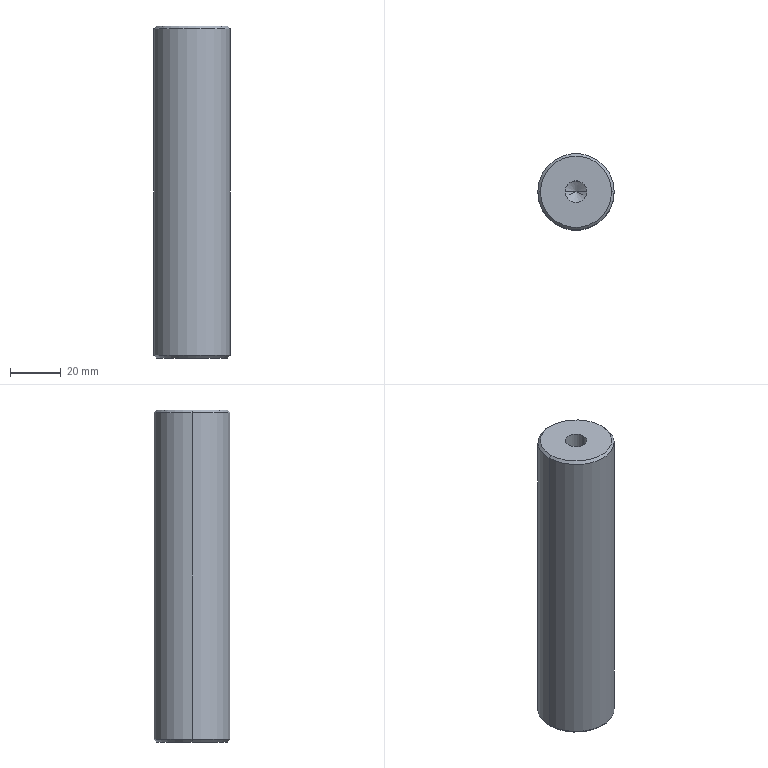Part | STEP file | LM-05-1254B_default | 1 solid | 16 faces | box 30 x 30 x 130.5 mm | volume 89786 mm3 | cone 8 | cylinder 6 | plane 2 | commonest cylinder face diameters 8.5 x4 30 x2
STEP:
#1=CARTESIAN_POINT('',(0.,0.,0.));
#2=DIRECTION('',(0.,0.,1.));
#3=DIRECTION('',(1.,0.,0.));
#4=AXIS2_PLACEMENT_3D('',#1,#2,#3);
#5=CARTESIAN_POINT('',(14.,0.,65.25));
#6=VERTEX_POINT('',#5);
#7=CARTESIAN_POINT('',(-14.,0.,65.25));
#8=VERTEX_POINT('',#7);
#9=CARTESIAN_POINT('',(0.,0.,65.25));
#10=DIRECTION('',(0.,0.,1.));
#11=DIRECTION('',(1.,0.,0.));
#12=AXIS2_PLACEMENT_3D('',#9,#10,#11);
#13=CIRCLE('',#12,14.);
#14=CARTESIAN_POINT('',(0.,0.,65.25));
#15=DIRECTION('',(0.,0.,-1.));
#16=DIRECTION('',(-1.,0.,0.));
#17=AXIS2_PLACEMENT_3D('',#14,#15,#16);
#18=CONICAL_SURFACE('',#17,14.,0.7854);
#19=CARTESIAN_POINT('',(3.142,0.));
#20=DIRECTION('',(-1.,0.));
#21=VECTOR('',#20,1.);
#22=LINE('',#19,#21);
#23=(GEOMETRIC_REPRESENTATION_CONTEXT(2)PARAMETRIC_REPRESENTATION_CONTEXT()REPRESENTATION_CONTEXT('',''));
#24=DEFINITIONAL_REPRESENTATION('',(#22),#23);
#25=PCURVE('',#18,#24);
#26=CARTESIAN_POINT('',(0.,0.,65.25));
#27=DIRECTION('',(0.,0.,1.));
#28=DIRECTION('',(1.,0.,0.));
#29=AXIS2_PLACEMENT_3D('',#26,#27,#28);
#30=PLANE('',#29);
#31=CARTESIAN_POINT('',(0.,0.));
#32=DIRECTION('',(1.,0.));
#33=AXIS2_PLACEMENT_2D('',#31,#32);
#34=CIRCLE('',#33,14.);
#35=(GEOMETRIC_REPRESENTATION_CONTEXT(2)PARAMETRIC_REPRESENTATION_CONTEXT()REPRESENTATION_CONTEXT('',''));
#36=DEFINITIONAL_REPRESENTATION('',(#34),#35);
#37=PCURVE('',#30,#36);
#38=SURFACE_CURVE('',#13,(#25,#37),.PCURVE_S1.);
#39=EDGE_CURVE('',#6,#8,#38,.T.);
#40=ORIENTED_EDGE('',*,*,#39,.F.);
#41=CARTESIAN_POINT('',(15.,0.,64.25));
#42=VERTEX_POINT('',#41);
#43=CARTESIAN_POINT('',(14.,0.,65.25));
#44=DIRECTION('',(0.7071,0.,-0.7071));
#45=VECTOR('',#44,1.);
#46=LINE('',#43,#45);
#47=CARTESIAN_POINT('',(3.142,0.));
#48=DIRECTION('',(0.,1.));
#49=VECTOR('',#48,1.);
#50=LINE('',#47,#49);
#51=(GEOMETRIC_REPRESENTATION_CONTEXT(2)PARAMETRIC_REPRESENTATION_CONTEXT()REPRESENTATION_CONTEXT('',''));
#52=DEFINITIONAL_REPRESENTATION('',(#50),#51);
#53=PCURVE('',#18,#52);
#54=CARTESIAN_POINT('',(0.,0.,65.25));
#55=DIRECTION('',(0.,0.,-1.));
#56=DIRECTION('',(-1.,0.,0.));
#57=AXIS2_PLACEMENT_3D('',#54,#55,#56);
#58=CONICAL_SURFACE('',#57,14.,0.7854);
#59=CARTESIAN_POINT('',(3.142,0.));
#60=DIRECTION('',(0.,1.));
#61=VECTOR('',#60,1.);
#62=LINE('',#59,#61);
#63=(GEOMETRIC_REPRESENTATION_CONTEXT(2)PARAMETRIC_REPRESENTATION_CONTEXT()REPRESENTATION_CONTEXT('',''));
#64=DEFINITIONAL_REPRESENTATION('',(#62),#63);
#65=PCURVE('',#58,#64);
#66=SURFACE_CURVE('',#46,(#53,#65),.PCURVE_S1.);
#67=EDGE_CURVE('',#6,#42,#66,.T.);
#68=ORIENTED_EDGE('',*,*,#67,.T.);
#69=CARTESIAN_POINT('',(-15.,0.,64.25));
#70=VERTEX_POINT('',#69);
#71=CARTESIAN_POINT('',(0.,0.,64.25));
#72=DIRECTION('',(0.,0.,-1.));
#73=DIRECTION('',(1.,0.,0.));
#74=AXIS2_PLACEMENT_3D('',#71,#72,#73);
#75=CIRCLE('',#74,15.);
#76=CARTESIAN_POINT('',(-3.142,1.));
#77=DIRECTION('',(1.,0.));
#78=VECTOR('',#77,1.);
#79=LINE('',#76,#78);
#80=(GEOMETRIC_REPRESENTATION_CONTEXT(2)PARAMETRIC_REPRESENTATION_CONTEXT()REPRESENTATION_CONTEXT('',''));
#81=DEFINITIONAL_REPRESENTATION('',(#79),#80);
#82=PCURVE('',#18,#81);
#83=CARTESIAN_POINT('',(0.,0.,65.25));
#84=DIRECTION('',(0.,0.,-1.));
#85=DIRECTION('',(-1.,0.,0.));
#86=AXIS2_PLACEMENT_3D('',#83,#84,#85);
#87=CYLINDRICAL_SURFACE('',#86,15.);
#88=CARTESIAN_POINT('',(-3.142,1.));
#89=DIRECTION('',(1.,0.));
#90=VECTOR('',#89,1.);
#91=LINE('',#88,#90);
#92=(GEOMETRIC_REPRESENTATION_CONTEXT(2)PARAMETRIC_REPRESENTATION_CONTEXT()REPRESENTATION_CONTEXT('',''));
#93=DEFINITIONAL_REPRESENTATION('',(#91),#92);
#94=PCURVE('',#87,#93);
#95=SURFACE_CURVE('',#75,(#82,#94),.PCURVE_S1.);
#96=EDGE_CURVE('',#70,#42,#95,.T.);
#97=ORIENTED_EDGE('',*,*,#96,.F.);
#98=CARTESIAN_POINT('',(-14.,0.,65.25));
#99=DIRECTION('',(-0.7071,0.,-0.7071));
#100=VECTOR('',#99,1.);
#101=LINE('',#98,#100);
#102=CARTESIAN_POINT('',(0.,0.));
#103=DIRECTION('',(0.,1.));
#104=VECTOR('',#103,1.);
#105=LINE('',#102,#104);
#106=(GEOMETRIC_REPRESENTATION_CONTEXT(2)PARAMETRIC_REPRESENTATION_CONTEXT()REPRESENTATION_CONTEXT('',''));
#107=DEFINITIONAL_REPRESENTATION('',(#105),#106);
#108=PCURVE('',#18,#107);
#109=CARTESIAN_POINT('',(6.283,0.));
#110=DIRECTION('',(0.,1.));
#111=VECTOR('',#110,1.);
#112=LINE('',#109,#111);
#113=(GEOMETRIC_REPRESENTATION_CONTEXT(2)PARAMETRIC_REPRESENTATION_CONTEXT()REPRESENTATION_CONTEXT('',''));
#114=DEFINITIONAL_REPRESENTATION('',(#112),#113);
#115=PCURVE('',#58,#114);
#116=SURFACE_CURVE('',#101,(#108,#115),.PCURVE_S1.);
#117=EDGE_CURVE('',#8,#70,#116,.T.);
#118=ORIENTED_EDGE('',*,*,#117,.F.);
#119=EDGE_LOOP('',(#40,#68,#97,#118));
#120=FACE_BOUND('',#119,.T.);
#121=ADVANCED_FACE('',(#120),#18,.T.);
#122=CARTESIAN_POINT('',(-14.,0.,-65.25));
#123=VERTEX_POINT('',#122);
#124=CARTESIAN_POINT('',(14.,0.,-65.25));
#125=VERTEX_POINT('',#124);
#126=CARTESIAN_POINT('',(0.,0.,-65.25));
#127=DIRECTION('',(0.,0.,-1.));
#128=DIRECTION('',(1.,0.,0.));
#129=AXIS2_PLACEMENT_3D('',#126,#127,#128);
#130=CIRCLE('',#129,14.);
#131=CARTESIAN_POINT('',(0.,0.,-64.25));
#132=DIRECTION('',(0.,0.,1.));
#133=DIRECTION('',(1.,0.,0.));
#134=AXIS2_PLACEMENT_3D('',#131,#132,#133);
#135=CONICAL_SURFACE('',#134,15.,0.7854);
#136=CARTESIAN_POINT('',(6.283,-1.));
#137=DIRECTION('',(-1.,0.));
#138=VECTOR('',#137,1.);
#139=LINE('',#136,#138);
#140=(GEOMETRIC_REPRESENTATION_CONTEXT(2)PARAMETRIC_REPRESENTATION_CONTEXT()REPRESENTATION_CONTEXT('',''));
#141=DEFINITIONAL_REPRESENTATION('',(#139),#140);
#142=PCURVE('',#135,#141);
#143=CARTESIAN_POINT('',(0.,0.,-65.25));
#144=DIRECTION('',(0.,0.,1.));
#145=DIRECTION('',(1.,0.,0.));
#146=AXIS2_PLACEMENT_3D('',#143,#144,#145);
#147=PLANE('',#146);
#148=CARTESIAN_POINT('',(14.,0.));
#149=CARTESIAN_POINT('',(14.,-24.249));
#150=CARTESIAN_POINT('',(-7.,-12.124));
#151=CARTESIAN_POINT('',(-28.,0.));
#152=CARTESIAN_POINT('',(-7.,12.124));
#153=CARTESIAN_POINT('',(14.,24.249));
#154=CARTESIAN_POINT('',(14.,0.));
#155=(BOUNDED_CURVE()B_SPLINE_CURVE(2,(#148,#149,#150,#151,#152,#153,#154),.UNSPECIFIED.,.T.,.F.)B_SPLINE_CURVE_WITH_KNOTS((1,2,2,2,2,1),(-2.094,0.,2.094,4.189,6.283,8.378),.UNSPECIFIED.)CURVE()GEOMETRIC_REPRESENTATION_ITEM()RATIONAL_B_SPLINE_CURVE((1.,0.5,1.,0.5,1.,0.5,1.))REPRESENTATION_ITEM(''));
#156=(GEOMETRIC_REPRESENTATION_CONTEXT(2)PARAMETRIC_REPRESENTATION_CONTEXT()REPRESENTATION_CONTEXT('',''));
#157=DEFINITIONAL_REPRESENTATION('',(#155),#156);
#158=PCURVE('',#147,#157);
#159=SURFACE_CURVE('',#130,(#142,#158),.PCURVE_S1.);
#160=EDGE_CURVE('',#123,#125,#159,.T.);
#161=ORIENTED_EDGE('',*,*,#160,.F.);
#162=CARTESIAN_POINT('',(-15.,0.,-64.25));
#163=VERTEX_POINT('',#162);
#164=CARTESIAN_POINT('',(-15.,0.,-64.25));
#165=DIRECTION('',(-0.7071,0.,0.7071));
#166=VECTOR('',#165,1.);
#167=LINE('',#164,#166);
#168=CARTESIAN_POINT('',(3.142,0.));
#169=DIRECTION('',(0.,1.));
#170=VECTOR('',#169,1.);
#171=LINE('',#168,#170);
#172=(GEOMETRIC_REPRESENTATION_CONTEXT(2)PARAMETRIC_REPRESENTATION_CONTEXT()REPRESENTATION_CONTEXT('',''));
#173=DEFINITIONAL_REPRESENTATION('',(#171),#172);
#174=PCURVE('',#135,#173);
#175=CARTESIAN_POINT('',(0.,0.,-64.25));
#176=DIRECTION('',(0.,0.,1.));
#177=DIRECTION('',(1.,0.,0.));
#178=AXIS2_PLACEMENT_3D('',#175,#176,#177);
#179=CONICAL_SURFACE('',#178,15.,0.7854);
#180=CARTESIAN_POINT('',(3.142,0.));
#181=DIRECTION('',(0.,1.));
#182=VECTOR('',#181,1.);
#183=LINE('',#180,#182);
#184=(GEOMETRIC_REPRESENTATION_CONTEXT(2)PARAMETRIC_REPRESENTATION_CONTEXT()REPRESENTATION_CONTEXT('',''));
#185=DEFINITIONAL_REPRESENTATION('',(#183),#184);
#186=PCURVE('',#179,#185);
#187=SURFACE_CURVE('',#167,(#174,#186),.PCURVE_S1.);
#188=EDGE_CURVE('',#123,#163,#187,.T.);
#189=ORIENTED_EDGE('',*,*,#188,.T.);
#190=CARTESIAN_POINT('',(15.,0.,-64.25));
#191=VERTEX_POINT('',#190);
#192=CARTESIAN_POINT('',(0.,0.,-64.25));
#193=DIRECTION('',(0.,0.,1.));
#194=DIRECTION('',(1.,0.,0.));
#195=AXIS2_PLACEMENT_3D('',#192,#193,#194);
#196=CIRCLE('',#195,15.);
#197=CARTESIAN_POINT('',(0.,0.));
#198=DIRECTION('',(1.,0.));
#199=VECTOR('',#198,1.);
#200=LINE('',#197,#199);
#201=(GEOMETRIC_REPRESENTATION_CONTEXT(2)PARAMETRIC_REPRESENTATION_CONTEXT()REPRESENTATION_CONTEXT('',''));
#202=DEFINITIONAL_REPRESENTATION('',(#200),#201);
#203=PCURVE('',#135,#202);
#204=CARTESIAN_POINT('',(3.142,129.5));
#205=DIRECTION('',(-1.,0.));
#206=VECTOR('',#205,1.);
#207=LINE('',#204,#206);
#208=(GEOMETRIC_REPRESENTATION_CONTEXT(2)PARAMETRIC_REPRESENTATION_CONTEXT()REPRESENTATION_CONTEXT('',''));
#209=DEFINITIONAL_REPRESENTATION('',(#207),#208);
#210=PCURVE('',#87,#209);
#211=SURFACE_CURVE('',#196,(#203,#210),.PCURVE_S1.);
#212=EDGE_CURVE('',#191,#163,#211,.T.);
#213=ORIENTED_EDGE('',*,*,#212,.F.);
#214=CARTESIAN_POINT('',(15.,0.,-64.25));
#215=DIRECTION('',(0.7071,0.,0.7071));
#216=VECTOR('',#215,1.);
#217=LINE('',#214,#216);
#218=CARTESIAN_POINT('',(0.,0.));
#219=DIRECTION('',(0.,1.));
#220=VECTOR('',#219,1.);
#221=LINE('',#218,#220);
#222=(GEOMETRIC_REPRESENTATION_CONTEXT(2)PARAMETRIC_REPRESENTATION_CONTEXT()REPRESENTATION_CONTEXT('',''));
#223=DEFINITIONAL_REPRESENTATION('',(#221),#222);
#224=PCURVE('',#135,#223);
#225=CARTESIAN_POINT('',(6.283,0.));
#226=DIRECTION('',(0.,1.));
#227=VECTOR('',#226,1.);
#228=LINE('',#225,#227);
#229=(GEOMETRIC_REPRESENTATION_CONTEXT(2)PARAMETRIC_REPRESENTATION_CONTEXT()REPRESENTATION_CONTEXT('',''));
#230=DEFINITIONAL_REPRESENTATION('',(#228),#229);
#231=PCURVE('',#179,#230);
#232=SURFACE_CURVE('',#217,(#224,#231),.PCURVE_S1.);
#233=EDGE_CURVE('',#125,#191,#232,.T.);
#234=ORIENTED_EDGE('',*,*,#233,.F.);
#235=EDGE_LOOP('',(#161,#189,#213,#234));
#236=FACE_BOUND('',#235,.T.);
#237=ADVANCED_FACE('',(#236),#135,.T.);
#238=CARTESIAN_POINT('',(-4.25,0.,-45.25));
#239=VERTEX_POINT('',#238);
#240=CARTESIAN_POINT('',(-4.25,0.,-65.25));
#241=VERTEX_POINT('',#240);
#242=CARTESIAN_POINT('',(-4.25,0.,-65.25));
#243=DIRECTION('',(0.,0.,-1.));
#244=VECTOR('',#243,1.);
#245=LINE('',#242,#244);
#246=CARTESIAN_POINT('',(0.,0.,-65.25));
#247=DIRECTION('',(0.,0.,-1.));
#248=DIRECTION('',(-1.,0.,0.));
#249=AXIS2_PLACEMENT_3D('',#246,#247,#248);
#250=CYLINDRICAL_SURFACE('',#249,4.25);
#251=CARTESIAN_POINT('',(6.283,0.));
#252=DIRECTION('',(0.,1.));
#253=VECTOR('',#252,1.);
#254=LINE('',#251,#253);
#255=(GEOMETRIC_REPRESENTATION_CONTEXT(2)PARAMETRIC_REPRESENTATION_CONTEXT()REPRESENTATION_CONTEXT('',''));
#256=DEFINITIONAL_REPRESENTATION('',(#254),#255);
#257=PCURVE('',#250,#256);
#258=CARTESIAN_POINT('',(0.,0.,-65.25));
#259=DIRECTION('',(0.,0.,-1.));
#260=DIRECTION('',(-1.,0.,0.));
#261=AXIS2_PLACEMENT_3D('',#258,#259,#260);
#262=CYLINDRICAL_SURFACE('',#261,4.25);
#263=CARTESIAN_POINT('',(0.,0.));
#264=DIRECTION('',(0.,1.));
#265=VECTOR('',#264,1.);
#266=LINE('',#263,#265);
#267=(GEOMETRIC_REPRESENTATION_CONTEXT(2)PARAMETRIC_REPRESENTATION_CONTEXT()REPRESENTATION_CONTEXT('',''));
#268=DEFINITIONAL_REPRESENTATION('',(#266),#267);
#269=PCURVE('',#262,#268);
#270=SURFACE_CURVE('',#245,(#257,#269),.PCURVE_S1.);
#271=EDGE_CURVE('',#239,#241,#270,.T.);
#272=ORIENTED_EDGE('',*,*,#271,.T.);
#273=CARTESIAN_POINT('',(4.25,0.,-65.25));
#274=VERTEX_POINT('',#273);
#275=CARTESIAN_POINT('',(0.,0.,-65.25));
#276=DIRECTION('',(0.,0.,-1.));
#277=DIRECTION('',(-1.,0.,0.));
#278=AXIS2_PLACEMENT_3D('',#275,#276,#277);
#279=CIRCLE('',#278,4.25);
#280=CARTESIAN_POINT('',(0.,0.));
#281=DIRECTION('',(1.,0.));
#282=VECTOR('',#281,1.);
#283=LINE('',#280,#282);
#284=(GEOMETRIC_REPRESENTATION_CONTEXT(2)PARAMETRIC_REPRESENTATION_CONTEXT()REPRESENTATION_CONTEXT('',''));
#285=DEFINITIONAL_REPRESENTATION('',(#283),#284);
#286=PCURVE('',#250,#285);
#287=CARTESIAN_POINT('',(-4.25,0.));
#288=CARTESIAN_POINT('',(-4.25,7.361));
#289=CARTESIAN_POINT('',(2.125,3.681));
#290=CARTESIAN_POINT('',(8.5,0.));
#291=CARTESIAN_POINT('',(2.125,-3.681));
#292=CARTESIAN_POINT('',(-4.25,-7.361));
#293=CARTESIAN_POINT('',(-4.25,0.));
#294=(BOUNDED_CURVE()B_SPLINE_CURVE(2,(#287,#288,#289,#290,#291,#292,#293),.UNSPECIFIED.,.T.,.F.)B_SPLINE_CURVE_WITH_KNOTS((1,2,2,2,2,1),(-2.094,0.,2.094,4.189,6.283,8.378),.UNSPECIFIED.)CURVE()GEOMETRIC_REPRESENTATION_ITEM()RATIONAL_B_SPLINE_CURVE((1.,0.5,1.,0.5,1.,0.5,1.))REPRESENTATION_ITEM(''));
#295=(GEOMETRIC_REPRESENTATION_CONTEXT(2)PARAMETRIC_REPRESENTATION_CONTEXT()REPRESENTATION_CONTEXT('',''));
#296=DEFINITIONAL_REPRESENTATION('',(#294),#295);
#297=PCURVE('',#147,#296);
#298=SURFACE_CURVE('',#279,(#286,#297),.PCURVE_S1.);
#299=EDGE_CURVE('',#274,#241,#298,.T.);
#300=ORIENTED_EDGE('',*,*,#299,.F.);
#301=CARTESIAN_POINT('',(4.25,0.,-45.25));
#302=VERTEX_POINT('',#301);
#303=CARTESIAN_POINT('',(4.25,0.,-65.25));
#304=DIRECTION('',(0.,0.,-1.));
#305=VECTOR('',#304,1.);
#306=LINE('',#303,#305);
#307=CARTESIAN_POINT('',(3.142,0.));
#308=DIRECTION('',(0.,1.));
#309=VECTOR('',#308,1.);
#310=LINE('',#307,#309);
#311=(GEOMETRIC_REPRESENTATION_CONTEXT(2)PARAMETRIC_REPRESENTATION_CONTEXT()REPRESENTATION_CONTEXT('',''));
#312=DEFINITIONAL_REPRESENTATION('',(#310),#311);
#313=PCURVE('',#250,#312);
#314=CARTESIAN_POINT('',(3.142,0.));
#315=DIRECTION('',(0.,1.));
#316=VECTOR('',#315,1.);
#317=LINE('',#314,#316);
#318=(GEOMETRIC_REPRESENTATION_CONTEXT(2)PARAMETRIC_REPRESENTATION_CONTEXT()REPRESENTATION_CONTEXT('',''));
#319=DEFINITIONAL_REPRESENTATION('',(#317),#318);
#320=PCURVE('',#262,#319);
#321=SURFACE_CURVE('',#306,(#313,#320),.PCURVE_S1.);
#322=EDGE_CURVE('',#302,#274,#321,.T.);
#323=ORIENTED_EDGE('',*,*,#322,.F.);
#324=CARTESIAN_POINT('',(0.,0.,-45.25));
#325=DIRECTION('',(0.,0.,-1.));
#326=DIRECTION('',(-1.,0.,0.));
#327=AXIS2_PLACEMENT_3D('',#324,#325,#326);
#328=CIRCLE('',#327,4.25);
#329=CARTESIAN_POINT('',(0.,-20.));
#330=DIRECTION('',(1.,0.));
#331=VECTOR('',#330,1.);
#332=LINE('',#329,#331);
#333=(GEOMETRIC_REPRESENTATION_CONTEXT(2)PARAMETRIC_REPRESENTATION_CONTEXT()REPRESENTATION_CONTEXT('',''));
#334=DEFINITIONAL_REPRESENTATION('',(#332),#333);
#335=PCURVE('',#250,#334);
#336=CARTESIAN_POINT('',(0.,0.,-45.25));
#337=DIRECTION('',(0.,0.,-1.));
#338=DIRECTION('',(-1.,0.,0.));
#339=AXIS2_PLACEMENT_3D('',#336,#337,#338);
#340=CONICAL_SURFACE('',#339,4.25,1.03);
#341=CARTESIAN_POINT('',(0.,0.));
#342=DIRECTION('',(1.,0.));
#343=VECTOR('',#342,1.);
#344=LINE('',#341,#343);
#345=(GEOMETRIC_REPRESENTATION_CONTEXT(2)PARAMETRIC_REPRESENTATION_CONTEXT()REPRESENTATION_CONTEXT('',''));
#346=DEFINITIONAL_REPRESENTATION('',(#344),#345);
#347=PCURVE('',#340,#346);
#348=SURFACE_CURVE('',#328,(#335,#347),.PCURVE_S1.);
#349=EDGE_CURVE('',#302,#239,#348,.T.);
#350=ORIENTED_EDGE('',*,*,#349,.T.);
#351=EDGE_LOOP('',(#272,#300,#323,#350));
#352=FACE_BOUND('',#351,.F.);
#353=ADVANCED_FACE('',(#352),#250,.F.);
#354=ORIENTED_EDGE('',*,*,#349,.F.);
#355=CARTESIAN_POINT('',(0.,0.,-42.696));
#356=VERTEX_POINT('',#355);
#357=CARTESIAN_POINT('',(4.25,0.,-45.25));
#358=DIRECTION('',(0.8572,0.,-0.515));
#359=VECTOR('',#358,1.);
#360=LINE('',#357,#359);
#361=CARTESIAN_POINT('',(3.142,0.));
#362=DIRECTION('',(0.,1.));
#363=VECTOR('',#362,1.);
#364=LINE('',#361,#363);
#365=(GEOMETRIC_REPRESENTATION_CONTEXT(2)PARAMETRIC_REPRESENTATION_CONTEXT()REPRESENTATION_CONTEXT('',''));
#366=DEFINITIONAL_REPRESENTATION('',(#364),#365);
#367=PCURVE('',#340,#366);
#368=CARTESIAN_POINT('',(0.,0.,-45.25));
#369=DIRECTION('',(0.,0.,-1.));
#370=DIRECTION('',(-1.,0.,0.));
#371=AXIS2_PLACEMENT_3D('',#368,#369,#370);
#372=CONICAL_SURFACE('',#371,4.25,1.03);
#373=CARTESIAN_POINT('',(3.142,0.));
#374=DIRECTION('',(0.,1.));
#375=VECTOR('',#374,1.);
#376=LINE('',#373,#375);
#377=(GEOMETRIC_REPRESENTATION_CONTEXT(2)PARAMETRIC_REPRESENTATION_CONTEXT()REPRESENTATION_CONTEXT('',''));
#378=DEFINITIONAL_REPRESENTATION('',(#376),#377);
#379=PCURVE('',#372,#378);
#380=SURFACE_CURVE('',#360,(#367,#379),.PCURVE_S1.);
#381=EDGE_CURVE('',#356,#302,#380,.T.);
#382=ORIENTED_EDGE('',*,*,#381,.F.);
#383=CARTESIAN_POINT('',(-4.25,0.,-45.25));
#384=DIRECTION('',(-0.8572,0.,-0.515));
#385=VECTOR('',#384,1.);
#386=LINE('',#383,#385);
#387=CARTESIAN_POINT('',(6.283,0.));
#388=DIRECTION('',(0.,1.));
#389=VECTOR('',#388,1.);
#390=LINE('',#387,#389);
#391=(GEOMETRIC_REPRESENTATION_CONTEXT(2)PARAMETRIC_REPRESENTATION_CONTEXT()REPRESENTATION_CONTEXT('',''));
#392=DEFINITIONAL_REPRESENTATION('',(#390),#391);
#393=PCURVE('',#340,#392);
#394=CARTESIAN_POINT('',(0.,0.));
#395=DIRECTION('',(0.,1.));
#396=VECTOR('',#395,1.);
#397=LINE('',#394,#396);
#398=(GEOMETRIC_REPRESENTATION_CONTEXT(2)PARAMETRIC_REPRESENTATION_CONTEXT()REPRESENTATION_CONTEXT('',''));
#399=DEFINITIONAL_REPRESENTATION('',(#397),#398);
#400=PCURVE('',#372,#399);
#401=SURFACE_CURVE('',#386,(#393,#400),.PCURVE_S1.);
#402=EDGE_CURVE('',#356,#239,#401,.T.);
#403=ORIENTED_EDGE('',*,*,#402,.T.);
#404=EDGE_LOOP('',(#354,#382,#403));
#405=FACE_BOUND('',#404,.F.);
#406=ADVANCED_FACE('',(#405),#340,.F.);
#407=CARTESIAN_POINT('',(4.25,0.,45.25));
#408=VERTEX_POINT('',#407);
#409=CARTESIAN_POINT('',(4.25,0.,65.25));
#410=VERTEX_POINT('',#409);
#411=CARTESIAN_POINT('',(4.25,0.,65.25));
#412=DIRECTION('',(0.,0.,1.));
#413=VECTOR('',#412,1.);
#414=LINE('',#411,#413);
#415=CARTESIAN_POINT('',(0.,0.,65.25));
#416=DIRECTION('',(0.,0.,1.));
#417=DIRECTION('',(1.,0.,0.));
#418=AXIS2_PLACEMENT_3D('',#415,#416,#417);
#419=CYLINDRICAL_SURFACE('',#418,4.25);
#420=CARTESIAN_POINT('',(6.283,0.));
#421=DIRECTION('',(0.,1.));
#422=VECTOR('',#421,1.);
#423=LINE('',#420,#422);
#424=(GEOMETRIC_REPRESENTATION_CONTEXT(2)PARAMETRIC_REPRESENTATION_CONTEXT()REPRESENTATION_CONTEXT('',''));
#425=DEFINITIONAL_REPRESENTATION('',(#423),#424);
#426=PCURVE('',#419,#425);
#427=CARTESIAN_POINT('',(0.,0.,65.25));
#428=DIRECTION('',(0.,0.,1.));
#429=DIRECTION('',(1.,0.,0.));
#430=AXIS2_PLACEMENT_3D('',#427,#428,#429);
#431=CYLINDRICAL_SURFACE('',#430,4.25);
#432=CARTESIAN_POINT('',(0.,0.));
#433=DIRECTION('',(0.,1.));
#434=VECTOR('',#433,1.);
#435=LINE('',#432,#434);
#436=(GEOMETRIC_REPRESENTATION_CONTEXT(2)PARAMETRIC_REPRESENTATION_CONTEXT()REPRESENTATION_CONTEXT('',''));
#437=DEFINITIONAL_REPRESENTATION('',(#435),#436);
#438=PCURVE('',#431,#437);
#439=SURFACE_CURVE('',#414,(#426,#438),.PCURVE_S1.);
#440=EDGE_CURVE('',#408,#410,#439,.T.);
#441=ORIENTED_EDGE('',*,*,#440,.T.);
#442=CARTESIAN_POINT('',(-4.25,0.,65.25));
#443=VERTEX_POINT('',#442);
#444=CARTESIAN_POINT('',(0.,0.,65.25));
#445=DIRECTION('',(0.,0.,1.));
#446=DIRECTION('',(1.,0.,0.));
#447=AXIS2_PLACEMENT_3D('',#444,#445,#446);
#448=CIRCLE('',#447,4.25);
#449=CARTESIAN_POINT('',(0.,0.));
#450=DIRECTION('',(1.,0.));
#451=VECTOR('',#450,1.);
#452=LINE('',#449,#451);
#453=(GEOMETRIC_REPRESENTATION_CONTEXT(2)PARAMETRIC_REPRESENTATION_CONTEXT()REPRESENTATION_CONTEXT('',''));
#454=DEFINITIONAL_REPRESENTATION('',(#452),#453);
#455=PCURVE('',#419,#454);
#456=CARTESIAN_POINT('',(0.,0.));
#457=DIRECTION('',(1.,0.));
#458=AXIS2_PLACEMENT_2D('',#456,#457);
#459=CIRCLE('',#458,4.25);
#460=(GEOMETRIC_REPRESENTATION_CONTEXT(2)PARAMETRIC_REPRESENTATION_CONTEXT()REPRESENTATION_CONTEXT('',''));
#461=DEFINITIONAL_REPRESENTATION('',(#459),#460);
#462=PCURVE('',#30,#461);
#463=SURFACE_CURVE('',#448,(#455,#462),.PCURVE_S1.);
#464=EDGE_CURVE('',#443,#410,#463,.T.);
#465=ORIENTED_EDGE('',*,*,#464,.F.);
#466=CARTESIAN_POINT('',(-4.25,0.,45.25));
#467=VERTEX_POINT('',#466);
#468=CARTESIAN_POINT('',(-4.25,0.,65.25));
#469=DIRECTION('',(0.,0.,1.));
#470=VECTOR('',#469,1.);
#471=LINE('',#468,#470);
#472=CARTESIAN_POINT('',(3.142,0.));
#473=DIRECTION('',(0.,1.));
#474=VECTOR('',#473,1.);
#475=LINE('',#472,#474);
#476=(GEOMETRIC_REPRESENTATION_CONTEXT(2)PARAMETRIC_REPRESENTATION_CONTEXT()REPRESENTATION_CONTEXT('',''));
#477=DEFINITIONAL_REPRESENTATION('',(#475),#476);
#478=PCURVE('',#419,#477);
#479=CARTESIAN_POINT('',(3.142,0.));
#480=DIRECTION('',(0.,1.));
#481=VECTOR('',#480,1.);
#482=LINE('',#479,#481);
#483=(GEOMETRIC_REPRESENTATION_CONTEXT(2)PARAMETRIC_REPRESENTATION_CONTEXT()REPRESENTATION_CONTEXT('',''));
#484=DEFINITIONAL_REPRESENTATION('',(#482),#483);
#485=PCURVE('',#431,#484);
#486=SURFACE_CURVE('',#471,(#478,#485),.PCURVE_S1.);
#487=EDGE_CURVE('',#467,#443,#486,.T.);
#488=ORIENTED_EDGE('',*,*,#487,.F.);
#489=CARTESIAN_POINT('',(0.,0.,45.25));
#490=DIRECTION('',(0.,0.,1.));
#491=DIRECTION('',(1.,0.,0.));
#492=AXIS2_PLACEMENT_3D('',#489,#490,#491);
#493=CIRCLE('',#492,4.25);
#494=CARTESIAN_POINT('',(0.,-20.));
#495=DIRECTION('',(1.,0.));
#496=VECTOR('',#495,1.);
#497=LINE('',#494,#496);
#498=(GEOMETRIC_REPRESENTATION_CONTEXT(2)PARAMETRIC_REPRESENTATION_CONTEXT()REPRESENTATION_CONTEXT('',''));
#499=DEFINITIONAL_REPRESENTATION('',(#497),#498);
#500=PCURVE('',#419,#499);
#501=CARTESIAN_POINT('',(0.,0.,45.25));
#502=DIRECTION('',(0.,0.,1.));
#503=DIRECTION('',(1.,0.,0.));
#504=AXIS2_PLACEMENT_3D('',#501,#502,#503);
#505=CONICAL_SURFACE('',#504,4.25,1.03);
#506=CARTESIAN_POINT('',(0.,0.));
#507=DIRECTION('',(1.,0.));
#508=VECTOR('',#507,1.);
#509=LINE('',#506,#508);
#510=(GEOMETRIC_REPRESENTATION_CONTEXT(2)PARAMETRIC_REPRESENTATION_CONTEXT()REPRESENTATION_CONTEXT('',''));
#511=DEFINITIONAL_REPRESENTATION('',(#509),#510);
#512=PCURVE('',#505,#511);
#513=SURFACE_CURVE('',#493,(#500,#512),.PCURVE_S1.);
#514=EDGE_CURVE('',#467,#408,#513,.T.);
#515=ORIENTED_EDGE('',*,*,#514,.T.);
#516=EDGE_LOOP('',(#441,#465,#488,#515));
#517=FACE_BOUND('',#516,.F.);
#518=ADVANCED_FACE('',(#517),#419,.F.);
#519=ORIENTED_EDGE('',*,*,#514,.F.);
#520=CARTESIAN_POINT('',(0.,0.,42.696));
#521=VERTEX_POINT('',#520);
#522=CARTESIAN_POINT('',(-4.25,0.,45.25));
#523=DIRECTION('',(-0.8572,0.,0.515));
#524=VECTOR('',#523,1.);
#525=LINE('',#522,#524);
#526=CARTESIAN_POINT('',(3.142,0.));
#527=DIRECTION('',(0.,1.));
#528=VECTOR('',#527,1.);
#529=LINE('',#526,#528);
#530=(GEOMETRIC_REPRESENTATION_CONTEXT(2)PARAMETRIC_REPRESENTATION_CONTEXT()REPRESENTATION_CONTEXT('',''));
#531=DEFINITIONAL_REPRESENTATION('',(#529),#530);
#532=PCURVE('',#505,#531);
#533=CARTESIAN_POINT('',(0.,0.,45.25));
#534=DIRECTION('',(0.,0.,1.));
#535=DIRECTION('',(1.,0.,0.));
#536=AXIS2_PLACEMENT_3D('',#533,#534,#535);
#537=CONICAL_SURFACE('',#536,4.25,1.03);
#538=CARTESIAN_POINT('',(3.142,0.));
#539=DIRECTION('',(0.,1.));
#540=VECTOR('',#539,1.);
#541=LINE('',#538,#540);
#542=(GEOMETRIC_REPRESENTATION_CONTEXT(2)PARAMETRIC_REPRESENTATION_CONTEXT()REPRESENTATION_CONTEXT('',''));
#543=DEFINITIONAL_REPRESENTATION('',(#541),#542);
#544=PCURVE('',#537,#543);
#545=SURFACE_CURVE('',#525,(#532,#544),.PCURVE_S1.);
#546=EDGE_CURVE('',#521,#467,#545,.T.);
#547=ORIENTED_EDGE('',*,*,#546,.F.);
#548=CARTESIAN_POINT('',(4.25,0.,45.25));
#549=DIRECTION('',(0.8572,0.,0.515));
#550=VECTOR('',#549,1.);
#551=LINE('',#548,#550);
#552=CARTESIAN_POINT('',(6.283,0.));
#553=DIRECTION('',(0.,1.));
#554=VECTOR('',#553,1.);
#555=LINE('',#552,#554);
#556=(GEOMETRIC_REPRESENTATION_CONTEXT(2)PARAMETRIC_REPRESENTATION_CONTEXT()REPRESENTATION_CONTEXT('',''));
#557=DEFINITIONAL_REPRESENTATION('',(#555),#556);
#558=PCURVE('',#505,#557);
#559=CARTESIAN_POINT('',(0.,0.));
#560=DIRECTION('',(0.,1.));
#561=VECTOR('',#560,1.);
#562=LINE('',#559,#561);
#563=(GEOMETRIC_REPRESENTATION_CONTEXT(2)PARAMETRIC_REPRESENTATION_CONTEXT()REPRESENTATION_CONTEXT('',''));
#564=DEFINITIONAL_REPRESENTATION('',(#562),#563);
#565=PCURVE('',#537,#564);
#566=SURFACE_CURVE('',#551,(#558,#565),.PCURVE_S1.);
#567=EDGE_CURVE('',#521,#408,#566,.T.);
#568=ORIENTED_EDGE('',*,*,#567,.T.);
#569=EDGE_LOOP('',(#519,#547,#568));
#570=FACE_BOUND('',#569,.F.);
#571=ADVANCED_FACE('',(#570),#505,.F.);
#572=ORIENTED_EDGE('',*,*,#96,.T.);
#573=CARTESIAN_POINT('',(15.,0.,65.25));
#574=DIRECTION('',(0.,0.,-1.));
#575=VECTOR('',#574,1.);
#576=LINE('',#573,#575);
#577=CARTESIAN_POINT('',(3.142,0.));
#578=DIRECTION('',(0.,1.));
#579=VECTOR('',#578,1.);
#580=LINE('',#577,#579);
#581=(GEOMETRIC_REPRESENTATION_CONTEXT(2)PARAMETRIC_REPRESENTATION_CONTEXT()REPRESENTATION_CONTEXT('',''));
#582=DEFINITIONAL_REPRESENTATION('',(#580),#581);
#583=PCURVE('',#87,#582);
#584=CARTESIAN_POINT('',(0.,0.,65.25));
#585=DIRECTION('',(0.,0.,-1.));
#586=DIRECTION('',(-1.,0.,0.));
#587=AXIS2_PLACEMENT_3D('',#584,#585,#586);
#588=CYLINDRICAL_SURFACE('',#587,15.);
#589=CARTESIAN_POINT('',(3.142,0.));
#590=DIRECTION('',(0.,1.));
#591=VECTOR('',#590,1.);
#592=LINE('',#589,#591);
#593=(GEOMETRIC_REPRESENTATION_CONTEXT(2)PARAMETRIC_REPRESENTATION_CONTEXT()REPRESENTATION_CONTEXT('',''));
#594=DEFINITIONAL_REPRESENTATION('',(#592),#593);
#595=PCURVE('',#588,#594);
#596=SURFACE_CURVE('',#576,(#583,#595),.PCURVE_S1.);
#597=EDGE_CURVE('',#42,#191,#596,.T.);
#598=ORIENTED_EDGE('',*,*,#597,.T.);
#599=ORIENTED_EDGE('',*,*,#212,.T.);
#600=CARTESIAN_POINT('',(-15.,0.,65.25));
#601=DIRECTION('',(0.,0.,-1.));
#602=VECTOR('',#601,1.);
#603=LINE('',#600,#602);
#604=CARTESIAN_POINT('',(0.,0.));
#605=DIRECTION('',(0.,1.));
#606=VECTOR('',#605,1.);
#607=LINE('',#604,#606);
#608=(GEOMETRIC_REPRESENTATION_CONTEXT(2)PARAMETRIC_REPRESENTATION_CONTEXT()REPRESENTATION_CONTEXT('',''));
#609=DEFINITIONAL_REPRESENTATION('',(#607),#608);
#610=PCURVE('',#87,#609);
#611=CARTESIAN_POINT('',(6.283,0.));
#612=DIRECTION('',(0.,1.));
#613=VECTOR('',#612,1.);
#614=LINE('',#611,#613);
#615=(GEOMETRIC_REPRESENTATION_CONTEXT(2)PARAMETRIC_REPRESENTATION_CONTEXT()REPRESENTATION_CONTEXT('',''));
#616=DEFINITIONAL_REPRESENTATION('',(#614),#615);
#617=PCURVE('',#588,#616);
#618=SURFACE_CURVE('',#603,(#610,#617),.PCURVE_S1.);
#619=EDGE_CURVE('',#70,#163,#618,.T.);
#620=ORIENTED_EDGE('',*,*,#619,.F.);
#621=EDGE_LOOP('',(#572,#598,#599,#620));
#622=FACE_BOUND('',#621,.T.);
#623=ADVANCED_FACE('',(#622),#87,.T.);
#624=ORIENTED_EDGE('',*,*,#597,.F.);
#625=CARTESIAN_POINT('',(0.,0.,64.25));
#626=DIRECTION('',(0.,0.,-1.));
#627=DIRECTION('',(1.,0.,0.));
#628=AXIS2_PLACEMENT_3D('',#625,#626,#627);
#629=CIRCLE('',#628,15.);
#630=CARTESIAN_POINT('',(3.142,1.));
#631=DIRECTION('',(1.,0.));
#632=VECTOR('',#631,1.);
#633=LINE('',#630,#632);
#634=(GEOMETRIC_REPRESENTATION_CONTEXT(2)PARAMETRIC_REPRESENTATION_CONTEXT()REPRESENTATION_CONTEXT('',''));
#635=DEFINITIONAL_REPRESENTATION('',(#633),#634);
#636=PCURVE('',#588,#635);
#637=CARTESIAN_POINT('',(3.142,1.));
#638=DIRECTION('',(1.,0.));
#639=VECTOR('',#638,1.);
#640=LINE('',#637,#639);
#641=(GEOMETRIC_REPRESENTATION_CONTEXT(2)PARAMETRIC_REPRESENTATION_CONTEXT()REPRESENTATION_CONTEXT('',''));
#642=DEFINITIONAL_REPRESENTATION('',(#640),#641);
#643=PCURVE('',#58,#642);
#644=SURFACE_CURVE('',#629,(#636,#643),.PCURVE_S1.);
#645=EDGE_CURVE('',#42,#70,#644,.T.);
#646=ORIENTED_EDGE('',*,*,#645,.T.);
#647=ORIENTED_EDGE('',*,*,#619,.T.);
#648=CARTESIAN_POINT('',(0.,0.,-64.25));
#649=DIRECTION('',(0.,0.,1.));
#650=DIRECTION('',(1.,0.,0.));
#651=AXIS2_PLACEMENT_3D('',#648,#649,#650);
#652=CIRCLE('',#651,15.);
#653=CARTESIAN_POINT('',(9.425,129.5));
#654=DIRECTION('',(-1.,0.));
#655=VECTOR('',#654,1.);
#656=LINE('',#653,#655);
#657=(GEOMETRIC_REPRESENTATION_CONTEXT(2)PARAMETRIC_REPRESENTATION_CONTEXT()REPRESENTATION_CONTEXT('',''));
#658=DEFINITIONAL_REPRESENTATION('',(#656),#657);
#659=PCURVE('',#588,#658);
#660=CARTESIAN_POINT('',(0.,0.));
#661=DIRECTION('',(1.,0.));
#662=VECTOR('',#661,1.);
#663=LINE('',#660,#662);
#664=(GEOMETRIC_REPRESENTATION_CONTEXT(2)PARAMETRIC_REPRESENTATION_CONTEXT()REPRESENTATION_CONTEXT('',''));
#665=DEFINITIONAL_REPRESENTATION('',(#663),#664);
#666=PCURVE('',#179,#665);
#667=SURFACE_CURVE('',#652,(#659,#666),.PCURVE_S1.);
#668=EDGE_CURVE('',#163,#191,#667,.T.);
#669=ORIENTED_EDGE('',*,*,#668,.T.);
#670=EDGE_LOOP('',(#624,#646,#647,#669));
#671=FACE_BOUND('',#670,.T.);
#672=ADVANCED_FACE('',(#671),#588,.T.);
#673=CARTESIAN_POINT('',(0.,0.,65.25));
#674=DIRECTION('',(0.,0.,1.));
#675=DIRECTION('',(1.,0.,0.));
#676=AXIS2_PLACEMENT_3D('',#673,#674,#675);
#677=CIRCLE('',#676,14.);
#678=CARTESIAN_POINT('',(0.,0.));
#679=DIRECTION('',(1.,0.));
#680=AXIS2_PLACEMENT_2D('',#678,#679);
#681=CIRCLE('',#680,14.);
#682=(GEOMETRIC_REPRESENTATION_CONTEXT(2)PARAMETRIC_REPRESENTATION_CONTEXT()REPRESENTATION_CONTEXT('',''));
#683=DEFINITIONAL_REPRESENTATION('',(#681),#682);
#684=PCURVE('',#30,#683);
#685=CARTESIAN_POINT('',(9.425,0.));
#686=DIRECTION('',(-1.,0.));
#687=VECTOR('',#686,1.);
#688=LINE('',#685,#687);
#689=(GEOMETRIC_REPRESENTATION_CONTEXT(2)PARAMETRIC_REPRESENTATION_CONTEXT()REPRESENTATION_CONTEXT('',''));
#690=DEFINITIONAL_REPRESENTATION('',(#688),#689);
#691=PCURVE('',#58,#690);
#692=SURFACE_CURVE('',#677,(#684,#691),.PCURVE_S1.);
#693=EDGE_CURVE('',#8,#6,#692,.T.);
#694=ORIENTED_EDGE('',*,*,#693,.T.);
#695=ORIENTED_EDGE('',*,*,#39,.T.);
#696=EDGE_LOOP('',(#694,#695));
#697=FACE_BOUND('',#696,.T.);
#698=CARTESIAN_POINT('',(0.,0.,65.25));
#699=DIRECTION('',(0.,0.,1.));
#700=DIRECTION('',(1.,0.,0.));
#701=AXIS2_PLACEMENT_3D('',#698,#699,#700);
#702=CIRCLE('',#701,4.25);
#703=CARTESIAN_POINT('',(0.,0.));
#704=DIRECTION('',(1.,0.));
#705=AXIS2_PLACEMENT_2D('',#703,#704);
#706=CIRCLE('',#705,4.25);
#707=(GEOMETRIC_REPRESENTATION_CONTEXT(2)PARAMETRIC_REPRESENTATION_CONTEXT()REPRESENTATION_CONTEXT('',''));
#708=DEFINITIONAL_REPRESENTATION('',(#706),#707);
#709=PCURVE('',#30,#708);
#710=CARTESIAN_POINT('',(0.,0.));
#711=DIRECTION('',(1.,0.));
#712=VECTOR('',#711,1.);
#713=LINE('',#710,#712);
#714=(GEOMETRIC_REPRESENTATION_CONTEXT(2)PARAMETRIC_REPRESENTATION_CONTEXT()REPRESENTATION_CONTEXT('',''));
#715=DEFINITIONAL_REPRESENTATION('',(#713),#714);
#716=PCURVE('',#431,#715);
#717=SURFACE_CURVE('',#702,(#709,#716),.PCURVE_S1.);
#718=EDGE_CURVE('',#410,#443,#717,.T.);
#719=ORIENTED_EDGE('',*,*,#718,.F.);
#720=ORIENTED_EDGE('',*,*,#464,.F.);
#721=EDGE_LOOP('',(#719,#720));
#722=FACE_BOUND('',#721,.T.);
#723=ADVANCED_FACE('',(#697,#722),#30,.T.);
#724=CARTESIAN_POINT('',(0.,0.,-65.25));
#725=DIRECTION('',(0.,0.,-1.));
#726=DIRECTION('',(1.,0.,0.));
#727=AXIS2_PLACEMENT_3D('',#724,#725,#726);
#728=CIRCLE('',#727,14.);
#729=CARTESIAN_POINT('',(14.,0.));
#730=CARTESIAN_POINT('',(14.,-24.249));
#731=CARTESIAN_POINT('',(-7.,-12.124));
#732=CARTESIAN_POINT('',(-28.,0.));
#733=CARTESIAN_POINT('',(-7.,12.124));
#734=CARTESIAN_POINT('',(14.,24.249));
#735=CARTESIAN_POINT('',(14.,0.));
#736=(BOUNDED_CURVE()B_SPLINE_CURVE(2,(#729,#730,#731,#732,#733,#734,#735),.UNSPECIFIED.,.T.,.F.)B_SPLINE_CURVE_WITH_KNOTS((1,2,2,2,2,1),(-2.094,0.,2.094,4.189,6.283,8.378),.UNSPECIFIED.)CURVE()GEOMETRIC_REPRESENTATION_ITEM()RATIONAL_B_SPLINE_CURVE((1.,0.5,1.,0.5,1.,0.5,1.))REPRESENTATION_ITEM(''));
#737=(GEOMETRIC_REPRESENTATION_CONTEXT(2)PARAMETRIC_REPRESENTATION_CONTEXT()REPRESENTATION_CONTEXT('',''));
#738=DEFINITIONAL_REPRESENTATION('',(#736),#737);
#739=PCURVE('',#147,#738);
#740=CARTESIAN_POINT('',(6.283,-1.));
#741=DIRECTION('',(-1.,0.));
#742=VECTOR('',#741,1.);
#743=LINE('',#740,#742);
#744=(GEOMETRIC_REPRESENTATION_CONTEXT(2)PARAMETRIC_REPRESENTATION_CONTEXT()REPRESENTATION_CONTEXT('',''));
#745=DEFINITIONAL_REPRESENTATION('',(#743),#744);
#746=PCURVE('',#179,#745);
#747=SURFACE_CURVE('',#728,(#739,#746),.PCURVE_S1.);
#748=EDGE_CURVE('',#125,#123,#747,.T.);
#749=ORIENTED_EDGE('',*,*,#748,.T.);
#750=ORIENTED_EDGE('',*,*,#160,.T.);
#751=EDGE_LOOP('',(#749,#750));
#752=FACE_BOUND('',#751,.T.);
#753=CARTESIAN_POINT('',(0.,0.,-65.25));
#754=DIRECTION('',(0.,0.,-1.));
#755=DIRECTION('',(-1.,0.,0.));
#756=AXIS2_PLACEMENT_3D('',#753,#754,#755);
#757=CIRCLE('',#756,4.25);
#758=CARTESIAN_POINT('',(-4.25,0.));
#759=CARTESIAN_POINT('',(-4.25,7.361));
#760=CARTESIAN_POINT('',(2.125,3.681));
#761=CARTESIAN_POINT('',(8.5,0.));
#762=CARTESIAN_POINT('',(2.125,-3.681));
#763=CARTESIAN_POINT('',(-4.25,-7.361));
#764=CARTESIAN_POINT('',(-4.25,0.));
#765=(BOUNDED_CURVE()B_SPLINE_CURVE(2,(#758,#759,#760,#761,#762,#763,#764),.UNSPECIFIED.,.T.,.F.)B_SPLINE_CURVE_WITH_KNOTS((1,2,2,2,2,1),(-2.094,0.,2.094,4.189,6.283,8.378),.UNSPECIFIED.)CURVE()GEOMETRIC_REPRESENTATION_ITEM()RATIONAL_B_SPLINE_CURVE((1.,0.5,1.,0.5,1.,0.5,1.))REPRESENTATION_ITEM(''));
#766=(GEOMETRIC_REPRESENTATION_CONTEXT(2)PARAMETRIC_REPRESENTATION_CONTEXT()REPRESENTATION_CONTEXT('',''));
#767=DEFINITIONAL_REPRESENTATION('',(#765),#766);
#768=PCURVE('',#147,#767);
#769=CARTESIAN_POINT('',(0.,0.));
#770=DIRECTION('',(1.,0.));
#771=VECTOR('',#770,1.);
#772=LINE('',#769,#771);
#773=(GEOMETRIC_REPRESENTATION_CONTEXT(2)PARAMETRIC_REPRESENTATION_CONTEXT()REPRESENTATION_CONTEXT('',''));
#774=DEFINITIONAL_REPRESENTATION('',(#772),#773);
#775=PCURVE('',#262,#774);
#776=SURFACE_CURVE('',#757,(#768,#775),.PCURVE_S1.);
#777=EDGE_CURVE('',#241,#274,#776,.T.);
#778=ORIENTED_EDGE('',*,*,#777,.F.);
#779=ORIENTED_EDGE('',*,*,#299,.F.);
#780=EDGE_LOOP('',(#778,#779));
#781=FACE_BOUND('',#780,.T.);
#782=ADVANCED_FACE('',(#752,#781),#147,.F.);
#783=CARTESIAN_POINT('',(0.,0.,45.25));
#784=DIRECTION('',(0.,0.,1.));
#785=DIRECTION('',(1.,0.,0.));
#786=AXIS2_PLACEMENT_3D('',#783,#784,#785);
#787=CIRCLE('',#786,4.25);
#788=CARTESIAN_POINT('',(0.,0.));
#789=DIRECTION('',(1.,0.));
#790=VECTOR('',#789,1.);
#791=LINE('',#788,#790);
#792=(GEOMETRIC_REPRESENTATION_CONTEXT(2)PARAMETRIC_REPRESENTATION_CONTEXT()REPRESENTATION_CONTEXT('',''));
#793=DEFINITIONAL_REPRESENTATION('',(#791),#792);
#794=PCURVE('',#537,#793);
#795=CARTESIAN_POINT('',(0.,-20.));
#796=DIRECTION('',(1.,0.));
#797=VECTOR('',#796,1.);
#798=LINE('',#795,#797);
#799=(GEOMETRIC_REPRESENTATION_CONTEXT(2)PARAMETRIC_REPRESENTATION_CONTEXT()REPRESENTATION_CONTEXT('',''));
#800=DEFINITIONAL_REPRESENTATION('',(#798),#799);
#801=PCURVE('',#431,#800);
#802=SURFACE_CURVE('',#787,(#794,#801),.PCURVE_S1.);
#803=EDGE_CURVE('',#408,#467,#802,.T.);
#804=ORIENTED_EDGE('',*,*,#803,.F.);
#805=ORIENTED_EDGE('',*,*,#567,.F.);
#806=ORIENTED_EDGE('',*,*,#546,.T.);
#807=EDGE_LOOP('',(#804,#805,#806));
#808=FACE_BOUND('',#807,.F.);
#809=ADVANCED_FACE('',(#808),#537,.F.);
#810=ORIENTED_EDGE('',*,*,#718,.F.);
#811=ORIENTED_EDGE('',*,*,#440,.F.);
#812=ORIENTED_EDGE('',*,*,#803,.T.);
#813=ORIENTED_EDGE('',*,*,#487,.T.);
#814=EDGE_LOOP('',(#810,#811,#812,#813));
#815=FACE_BOUND('',#814,.F.);
#816=ADVANCED_FACE('',(#815),#431,.F.);
#817=CARTESIAN_POINT('',(0.,0.,-45.25));
#818=DIRECTION('',(0.,0.,-1.));
#819=DIRECTION('',(-1.,0.,0.));
#820=AXIS2_PLACEMENT_3D('',#817,#818,#819);
#821=CIRCLE('',#820,4.25);
#822=CARTESIAN_POINT('',(0.,0.));
#823=DIRECTION('',(1.,0.));
#824=VECTOR('',#823,1.);
#825=LINE('',#822,#824);
#826=(GEOMETRIC_REPRESENTATION_CONTEXT(2)PARAMETRIC_REPRESENTATION_CONTEXT()REPRESENTATION_CONTEXT('',''));
#827=DEFINITIONAL_REPRESENTATION('',(#825),#826);
#828=PCURVE('',#372,#827);
#829=CARTESIAN_POINT('',(0.,-20.));
#830=DIRECTION('',(1.,0.));
#831=VECTOR('',#830,1.);
#832=LINE('',#829,#831);
#833=(GEOMETRIC_REPRESENTATION_CONTEXT(2)PARAMETRIC_REPRESENTATION_CONTEXT()REPRESENTATION_CONTEXT('',''));
#834=DEFINITIONAL_REPRESENTATION('',(#832),#833);
#835=PCURVE('',#262,#834);
#836=SURFACE_CURVE('',#821,(#828,#835),.PCURVE_S1.);
#837=EDGE_CURVE('',#239,#302,#836,.T.);
#838=ORIENTED_EDGE('',*,*,#837,.F.);
#839=ORIENTED_EDGE('',*,*,#402,.F.);
#840=ORIENTED_EDGE('',*,*,#381,.T.);
#841=EDGE_LOOP('',(#838,#839,#840));
#842=FACE_BOUND('',#841,.F.);
#843=ADVANCED_FACE('',(#842),#372,.F.);
#844=ORIENTED_EDGE('',*,*,#777,.F.);
#845=ORIENTED_EDGE('',*,*,#271,.F.);
#846=ORIENTED_EDGE('',*,*,#837,.T.);
#847=ORIENTED_EDGE('',*,*,#322,.T.);
#848=EDGE_LOOP('',(#844,#845,#846,#847));
#849=FACE_BOUND('',#848,.F.);
#850=ADVANCED_FACE('',(#849),#262,.F.);
#851=ORIENTED_EDGE('',*,*,#188,.F.);
#852=ORIENTED_EDGE('',*,*,#748,.F.);
#853=ORIENTED_EDGE('',*,*,#233,.T.);
#854=ORIENTED_EDGE('',*,*,#668,.F.);
#855=EDGE_LOOP('',(#851,#852,#853,#854));
#856=FACE_BOUND('',#855,.T.);
#857=ADVANCED_FACE('',(#856),#179,.T.);
#858=ORIENTED_EDGE('',*,*,#67,.F.);
#859=ORIENTED_EDGE('',*,*,#693,.F.);
#860=ORIENTED_EDGE('',*,*,#117,.T.);
#861=ORIENTED_EDGE('',*,*,#645,.F.);
#862=EDGE_LOOP('',(#858,#859,#860,#861));
#863=FACE_BOUND('',#862,.T.);
#864=ADVANCED_FACE('',(#863),#58,.T.);
#865=CLOSED_SHELL('',(#121,#237,#353,#406,#518,#571,#623,#672,#723,#782,#809,#816,#843,#850,#857,#864));
#866=MANIFOLD_SOLID_BREP('',#865);
#867=(LENGTH_UNIT()NAMED_UNIT(*)SI_UNIT(.MILLI.,.METRE.));
#868=UNCERTAINTY_MEASURE_WITH_UNIT(LENGTH_MEASURE(0.0000001),#867,'','');
#869=(NAMED_UNIT(*)PLANE_ANGLE_UNIT()SI_UNIT($,.RADIAN.));
#870=(NAMED_UNIT(*)SI_UNIT($,.STERADIAN.)SOLID_ANGLE_UNIT());
#871=(GEOMETRIC_REPRESENTATION_CONTEXT(3)GLOBAL_UNCERTAINTY_ASSIGNED_CONTEXT((#868))GLOBAL_UNIT_ASSIGNED_CONTEXT((#867,#869,#870))REPRESENTATION_CONTEXT('',''));
#872=ADVANCED_BREP_SHAPE_REPRESENTATION('',(#4,#866),#871);